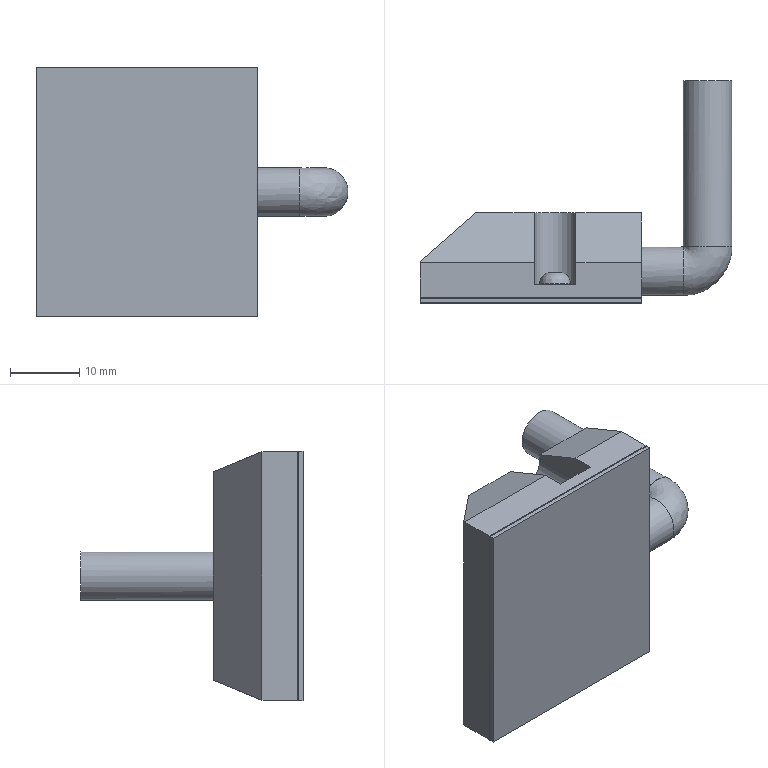Part | NX | 1 solid | 45 faces | box 45.035 x 32.1 x 36 mm | volume 14146 mm3 | plane 35 | cylinder 7 | spline 3 | commonest cylinder face diameters 4.5 x2 6 x2 7 x2 7.2 x1
STEP:
#1=CARTESIAN_POINT('',(-52.2,40.,-18.));
#2=VERTEX_POINT('',#1);
#3=CARTESIAN_POINT('',(-52.2,40.,18.));
#4=VERTEX_POINT('',#3);
#5=CARTESIAN_POINT('',(-52.2,40.,18.));
#6=DIRECTION('',(0.,0.,-1.));
#7=VECTOR('',#6,1000.);
#8=LINE('',#5,#7);
#9=EDGE_CURVE('',#2,#4,#8,.F.);
#10=ORIENTED_EDGE('',*,*,#9,.T.);
#11=CARTESIAN_POINT('',(-84.2,40.,18.));
#12=VERTEX_POINT('',#11);
#13=CARTESIAN_POINT('',(-52.2,40.,18.));
#14=DIRECTION('',(1.,0.,0.));
#15=VECTOR('',#14,1000.);
#16=LINE('',#13,#15);
#17=EDGE_CURVE('',#4,#12,#16,.F.);
#18=ORIENTED_EDGE('',*,*,#17,.T.);
#19=CARTESIAN_POINT('',(-84.2,40.,-18.));
#20=VERTEX_POINT('',#19);
#21=CARTESIAN_POINT('',(-84.2,40.,18.));
#22=DIRECTION('',(0.,0.,-1.));
#23=VECTOR('',#22,1000.);
#24=LINE('',#21,#23);
#25=EDGE_CURVE('',#12,#20,#24,.T.);
#26=ORIENTED_EDGE('',*,*,#25,.T.);
#27=CARTESIAN_POINT('',(-52.2,40.,-18.));
#28=DIRECTION('',(1.,0.,0.));
#29=VECTOR('',#28,1000.);
#30=LINE('',#27,#29);
#31=EDGE_CURVE('',#20,#2,#30,.T.);
#32=ORIENTED_EDGE('',*,*,#31,.T.);
#33=EDGE_LOOP('',(#10,#18,#26,#32));
#34=FACE_BOUND('',#33,.T.);
#35=CARTESIAN_POINT('',(-52.2,40.,18.));
#36=DIRECTION('',(0.,-1.,0.));
#37=DIRECTION('',(0.,0.,-1.));
#38=AXIS2_PLACEMENT_3D('',#35,#36,#37);
#39=PLANE('',#38);
#40=ADVANCED_FACE('',(#34),#39,.T.);
#41=CARTESIAN_POINT('',(-52.2,40.7,18.));
#42=VERTEX_POINT('',#41);
#43=CARTESIAN_POINT('',(-52.2,40.7,18.));
#44=DIRECTION('',(0.,1.,0.));
#45=VECTOR('',#44,1000.);
#46=LINE('',#43,#45);
#47=EDGE_CURVE('',#4,#42,#46,.T.);
#48=ORIENTED_EDGE('',*,*,#47,.T.);
#49=CARTESIAN_POINT('',(-84.2,40.7,18.));
#50=VERTEX_POINT('',#49);
#51=CARTESIAN_POINT('',(-52.2,40.7,18.));
#52=DIRECTION('',(1.,0.,0.));
#53=VECTOR('',#52,1000.);
#54=LINE('',#51,#53);
#55=EDGE_CURVE('',#42,#50,#54,.F.);
#56=ORIENTED_EDGE('',*,*,#55,.T.);
#57=CARTESIAN_POINT('',(-84.2,40.7,18.));
#58=DIRECTION('',(0.,1.,0.));
#59=VECTOR('',#58,1000.);
#60=LINE('',#57,#59);
#61=EDGE_CURVE('',#50,#12,#60,.F.);
#62=ORIENTED_EDGE('',*,*,#61,.T.);
#63=ORIENTED_EDGE('',*,*,#17,.F.);
#64=EDGE_LOOP('',(#48,#56,#62,#63));
#65=FACE_BOUND('',#64,.T.);
#66=CARTESIAN_POINT('',(-52.2,40.7,18.));
#67=DIRECTION('',(0.,0.,1.));
#68=DIRECTION('',(1.,0.,0.));
#69=AXIS2_PLACEMENT_3D('',#66,#67,#68);
#70=PLANE('',#69);
#71=ADVANCED_FACE('',(#65),#70,.T.);
#72=ORIENTED_EDGE('',*,*,#47,.F.);
#73=ORIENTED_EDGE('',*,*,#9,.F.);
#74=CARTESIAN_POINT('',(-52.2,40.7,-18.));
#75=VERTEX_POINT('',#74);
#76=CARTESIAN_POINT('',(-52.2,40.,-18.));
#77=DIRECTION('',(0.,1.,0.));
#78=VECTOR('',#77,1000.);
#79=LINE('',#76,#78);
#80=EDGE_CURVE('',#75,#2,#79,.F.);
#81=ORIENTED_EDGE('',*,*,#80,.F.);
#82=CARTESIAN_POINT('',(-52.2,40.7,0.));
#83=DIRECTION('',(0.,0.,1.));
#84=VECTOR('',#83,1000.);
#85=LINE('',#82,#84);
#86=EDGE_CURVE('',#42,#75,#85,.F.);
#87=ORIENTED_EDGE('',*,*,#86,.F.);
#88=EDGE_LOOP('',(#72,#73,#81,#87));
#89=FACE_BOUND('',#88,.T.);
#90=CARTESIAN_POINT('',(-52.2,40.,0.));
#91=DIRECTION('',(-1.,0.,0.));
#92=DIRECTION('',(0.,0.,1.));
#93=AXIS2_PLACEMENT_3D('',#90,#91,#92);
#94=PLANE('',#93);
#95=ADVANCED_FACE('',(#89),#94,.F.);
#96=ORIENTED_EDGE('',*,*,#80,.T.);
#97=ORIENTED_EDGE('',*,*,#31,.F.);
#98=CARTESIAN_POINT('',(-84.2,40.7,-18.));
#99=VERTEX_POINT('',#98);
#100=CARTESIAN_POINT('',(-84.2,40.,-18.));
#101=DIRECTION('',(0.,1.,0.));
#102=VECTOR('',#101,1000.);
#103=LINE('',#100,#102);
#104=EDGE_CURVE('',#20,#99,#103,.T.);
#105=ORIENTED_EDGE('',*,*,#104,.T.);
#106=CARTESIAN_POINT('',(-52.2,40.7,-18.));
#107=DIRECTION('',(-1.,0.,0.));
#108=VECTOR('',#107,1000.);
#109=LINE('',#106,#108);
#110=EDGE_CURVE('',#99,#75,#109,.F.);
#111=ORIENTED_EDGE('',*,*,#110,.T.);
#112=EDGE_LOOP('',(#96,#97,#105,#111));
#113=FACE_BOUND('',#112,.T.);
#114=CARTESIAN_POINT('',(-52.2,40.,-18.));
#115=DIRECTION('',(0.,0.,-1.));
#116=DIRECTION('',(-1.,0.,0.));
#117=AXIS2_PLACEMENT_3D('',#114,#115,#116);
#118=PLANE('',#117);
#119=ADVANCED_FACE('',(#113),#118,.T.);
#120=ORIENTED_EDGE('',*,*,#25,.F.);
#121=ORIENTED_EDGE('',*,*,#61,.F.);
#122=CARTESIAN_POINT('',(-84.2,40.7,0.));
#123=DIRECTION('',(0.,0.,1.));
#124=VECTOR('',#123,1000.);
#125=LINE('',#122,#124);
#126=EDGE_CURVE('',#50,#99,#125,.F.);
#127=ORIENTED_EDGE('',*,*,#126,.T.);
#128=ORIENTED_EDGE('',*,*,#104,.F.);
#129=EDGE_LOOP('',(#120,#121,#127,#128));
#130=FACE_BOUND('',#129,.T.);
#131=CARTESIAN_POINT('',(-84.2,40.,0.));
#132=DIRECTION('',(-1.,0.,0.));
#133=DIRECTION('',(0.,0.,1.));
#134=AXIS2_PLACEMENT_3D('',#131,#132,#133);
#135=PLANE('',#134);
#136=ADVANCED_FACE('',(#130),#135,.T.);
#137=ORIENTED_EDGE('',*,*,#86,.T.);
#138=ORIENTED_EDGE('',*,*,#110,.F.);
#139=ORIENTED_EDGE('',*,*,#126,.F.);
#140=ORIENTED_EDGE('',*,*,#55,.F.);
#141=EDGE_LOOP('',(#137,#138,#139,#140));
#142=FACE_BOUND('',#141,.T.);
#143=CARTESIAN_POINT('',(-52.3,40.7,17.9));
#144=VERTEX_POINT('',#143);
#145=CARTESIAN_POINT('',(-84.1,40.7,17.9));
#146=VERTEX_POINT('',#145);
#147=CARTESIAN_POINT('',(-52.2,40.7,17.9));
#148=DIRECTION('',(1.,0.,0.));
#149=VECTOR('',#148,1000.);
#150=LINE('',#147,#149);
#151=EDGE_CURVE('',#144,#146,#150,.F.);
#152=ORIENTED_EDGE('',*,*,#151,.T.);
#153=CARTESIAN_POINT('',(-84.1,40.7,-17.9));
#154=VERTEX_POINT('',#153);
#155=CARTESIAN_POINT('',(-84.1,40.7,-18.));
#156=DIRECTION('',(0.,0.,1.));
#157=VECTOR('',#156,1000.);
#158=LINE('',#155,#157);
#159=EDGE_CURVE('',#146,#154,#158,.F.);
#160=ORIENTED_EDGE('',*,*,#159,.T.);
#161=CARTESIAN_POINT('',(-52.3,40.7,-17.9));
#162=VERTEX_POINT('',#161);
#163=CARTESIAN_POINT('',(-52.2,40.7,-17.9));
#164=DIRECTION('',(1.,0.,0.));
#165=VECTOR('',#164,1000.);
#166=LINE('',#163,#165);
#167=EDGE_CURVE('',#154,#162,#166,.T.);
#168=ORIENTED_EDGE('',*,*,#167,.T.);
#169=CARTESIAN_POINT('',(-52.3,40.7,-18.));
#170=DIRECTION('',(0.,0.,1.));
#171=VECTOR('',#170,1000.);
#172=LINE('',#169,#171);
#173=EDGE_CURVE('',#162,#144,#172,.T.);
#174=ORIENTED_EDGE('',*,*,#173,.T.);
#175=EDGE_LOOP('',(#152,#160,#168,#174));
#176=FACE_BOUND('',#175,.T.);
#177=CARTESIAN_POINT('',(-52.2,40.7,-18.));
#178=DIRECTION('',(0.,1.,0.));
#179=DIRECTION('',(0.,0.,1.));
#180=AXIS2_PLACEMENT_3D('',#177,#178,#179);
#181=PLANE('',#180);
#182=ADVANCED_FACE('',(#142,#176),#181,.T.);
#183=CARTESIAN_POINT('',(-84.1,40.8,17.9));
#184=VERTEX_POINT('',#183);
#185=CARTESIAN_POINT('',(-84.1,40.,17.9));
#186=DIRECTION('',(0.,1.,0.));
#187=VECTOR('',#186,1000.);
#188=LINE('',#185,#187);
#189=EDGE_CURVE('',#146,#184,#188,.T.);
#190=ORIENTED_EDGE('',*,*,#189,.T.);
#191=CARTESIAN_POINT('',(-84.1,40.8,-17.9));
#192=VERTEX_POINT('',#191);
#193=CARTESIAN_POINT('',(-84.1,40.8,0.));
#194=DIRECTION('',(0.,0.,1.));
#195=VECTOR('',#194,1000.);
#196=LINE('',#193,#195);
#197=EDGE_CURVE('',#184,#192,#196,.F.);
#198=ORIENTED_EDGE('',*,*,#197,.T.);
#199=CARTESIAN_POINT('',(-84.1,40.,-17.9));
#200=DIRECTION('',(0.,1.,0.));
#201=VECTOR('',#200,1000.);
#202=LINE('',#199,#201);
#203=EDGE_CURVE('',#192,#154,#202,.F.);
#204=ORIENTED_EDGE('',*,*,#203,.T.);
#205=ORIENTED_EDGE('',*,*,#159,.F.);
#206=EDGE_LOOP('',(#190,#198,#204,#205));
#207=FACE_BOUND('',#206,.T.);
#208=CARTESIAN_POINT('',(-84.1,40.,0.));
#209=DIRECTION('',(-1.,0.,0.));
#210=DIRECTION('',(0.,0.,1.));
#211=AXIS2_PLACEMENT_3D('',#208,#209,#210);
#212=PLANE('',#211);
#213=ADVANCED_FACE('',(#207),#212,.T.);
#214=CARTESIAN_POINT('',(-52.3,40.8,17.9));
#215=VERTEX_POINT('',#214);
#216=CARTESIAN_POINT('',(-52.3,40.8,17.9));
#217=DIRECTION('',(0.,1.,0.));
#218=VECTOR('',#217,1000.);
#219=LINE('',#216,#218);
#220=EDGE_CURVE('',#144,#215,#219,.T.);
#221=ORIENTED_EDGE('',*,*,#220,.T.);
#222=CARTESIAN_POINT('',(-52.2,40.8,17.9));
#223=DIRECTION('',(1.,0.,0.));
#224=VECTOR('',#223,1000.);
#225=LINE('',#222,#224);
#226=EDGE_CURVE('',#215,#184,#225,.F.);
#227=ORIENTED_EDGE('',*,*,#226,.T.);
#228=ORIENTED_EDGE('',*,*,#189,.F.);
#229=ORIENTED_EDGE('',*,*,#151,.F.);
#230=EDGE_LOOP('',(#221,#227,#228,#229));
#231=FACE_BOUND('',#230,.T.);
#232=CARTESIAN_POINT('',(-52.2,40.8,17.9));
#233=DIRECTION('',(0.,0.,1.));
#234=DIRECTION('',(1.,0.,0.));
#235=AXIS2_PLACEMENT_3D('',#232,#233,#234);
#236=PLANE('',#235);
#237=ADVANCED_FACE('',(#231),#236,.T.);
#238=CARTESIAN_POINT('',(-52.3,40.8,-3.6));
#239=VERTEX_POINT('',#238);
#240=CARTESIAN_POINT('',(-52.3,40.8,-17.9));
#241=VERTEX_POINT('',#240);
#242=CARTESIAN_POINT('',(-52.3,40.8,0.));
#243=DIRECTION('',(0.,0.,1.));
#244=VECTOR('',#243,1000.);
#245=LINE('',#242,#244);
#246=EDGE_CURVE('',#239,#241,#245,.F.);
#247=ORIENTED_EDGE('',*,*,#246,.F.);
#248=CARTESIAN_POINT('',(-52.3,44.6,-3.6));
#249=VERTEX_POINT('',#248);
#250=CARTESIAN_POINT('',(-52.3,40.,-3.6));
#251=DIRECTION('',(0.,1.,0.));
#252=VECTOR('',#251,1000.);
#253=LINE('',#250,#252);
#254=EDGE_CURVE('',#249,#239,#253,.F.);
#255=ORIENTED_EDGE('',*,*,#254,.F.);
#256=CARTESIAN_POINT('',(-52.3,44.6,3.6));
#257=VERTEX_POINT('',#256);
#258=CARTESIAN_POINT('',(-52.3,44.6,0.));
#259=DIRECTION('',(1.,0.,0.));
#260=DIRECTION('',(0.,0.,-1.));
#261=AXIS2_PLACEMENT_3D('',#258,#259,#260);
#262=CIRCLE('',#261,3.6);
#263=EDGE_CURVE('',#257,#249,#262,.F.);
#264=ORIENTED_EDGE('',*,*,#263,.F.);
#265=CARTESIAN_POINT('',(-52.3,40.8,3.6));
#266=VERTEX_POINT('',#265);
#267=CARTESIAN_POINT('',(-52.3,40.,3.6));
#268=DIRECTION('',(0.,1.,0.));
#269=VECTOR('',#268,1000.);
#270=LINE('',#267,#269);
#271=EDGE_CURVE('',#266,#257,#270,.T.);
#272=ORIENTED_EDGE('',*,*,#271,.F.);
#273=CARTESIAN_POINT('',(-52.3,40.8,0.));
#274=DIRECTION('',(0.,0.,1.));
#275=VECTOR('',#274,1000.);
#276=LINE('',#273,#275);
#277=EDGE_CURVE('',#215,#266,#276,.F.);
#278=ORIENTED_EDGE('',*,*,#277,.F.);
#279=ORIENTED_EDGE('',*,*,#220,.F.);
#280=ORIENTED_EDGE('',*,*,#173,.F.);
#281=CARTESIAN_POINT('',(-52.3,40.,-17.9));
#282=DIRECTION('',(0.,1.,0.));
#283=VECTOR('',#282,1000.);
#284=LINE('',#281,#283);
#285=EDGE_CURVE('',#241,#162,#284,.F.);
#286=ORIENTED_EDGE('',*,*,#285,.F.);
#287=EDGE_LOOP('',(#247,#255,#264,#272,#278,#279,#280,#286));
#288=FACE_BOUND('',#287,.T.);
#289=CARTESIAN_POINT('',(-52.3,44.6,-3.5));
#290=VERTEX_POINT('',#289);
#291=CARTESIAN_POINT('',(-52.3,44.6,0.));
#292=DIRECTION('',(1.,0.,0.));
#293=DIRECTION('',(0.,0.,-1.));
#294=AXIS2_PLACEMENT_3D('',#291,#292,#293);
#295=CIRCLE('',#294,3.5);
#296=EDGE_CURVE('',#290,#290,#295,.T.);
#297=ORIENTED_EDGE('',*,*,#296,.F.);
#298=EDGE_LOOP('',(#297));
#299=FACE_BOUND('',#298,.T.);
#300=CARTESIAN_POINT('',(-52.3,40.,0.));
#301=DIRECTION('',(-1.,0.,0.));
#302=DIRECTION('',(0.,0.,1.));
#303=AXIS2_PLACEMENT_3D('',#300,#301,#302);
#304=PLANE('',#303);
#305=ADVANCED_FACE('',(#288,#299),#304,.F.);
#306=ORIENTED_EDGE('',*,*,#285,.T.);
#307=ORIENTED_EDGE('',*,*,#167,.F.);
#308=ORIENTED_EDGE('',*,*,#203,.F.);
#309=CARTESIAN_POINT('',(-52.2,40.8,-17.9));
#310=DIRECTION('',(1.,0.,0.));
#311=VECTOR('',#310,1000.);
#312=LINE('',#309,#311);
#313=EDGE_CURVE('',#192,#241,#312,.T.);
#314=ORIENTED_EDGE('',*,*,#313,.T.);
#315=EDGE_LOOP('',(#306,#307,#308,#314));
#316=FACE_BOUND('',#315,.T.);
#317=CARTESIAN_POINT('',(-52.2,40.7,-17.9));
#318=DIRECTION('',(0.,0.,-1.));
#319=DIRECTION('',(0.,1.,0.));
#320=AXIS2_PLACEMENT_3D('',#317,#318,#319);
#321=PLANE('',#320);
#322=ADVANCED_FACE('',(#316),#321,.T.);
#323=CARTESIAN_POINT('',(-84.2,40.8,-18.));
#324=VERTEX_POINT('',#323);
#325=CARTESIAN_POINT('',(-52.2,40.8,-18.));
#326=VERTEX_POINT('',#325);
#327=CARTESIAN_POINT('',(-52.2,40.8,-18.));
#328=DIRECTION('',(1.,0.,0.));
#329=VECTOR('',#328,1000.);
#330=LINE('',#327,#329);
#331=EDGE_CURVE('',#324,#326,#330,.T.);
#332=ORIENTED_EDGE('',*,*,#331,.T.);
#333=CARTESIAN_POINT('',(-52.2,40.8,-3.6));
#334=VERTEX_POINT('',#333);
#335=CARTESIAN_POINT('',(-52.2,40.8,-17.9));
#336=DIRECTION('',(0.,0.,-1.));
#337=VECTOR('',#336,1000.);
#338=LINE('',#335,#337);
#339=EDGE_CURVE('',#326,#334,#338,.F.);
#340=ORIENTED_EDGE('',*,*,#339,.T.);
#341=CARTESIAN_POINT('',(-52.2,40.8,-3.6));
#342=DIRECTION('',(1.,0.,0.));
#343=VECTOR('',#342,1000.);
#344=LINE('',#341,#343);
#345=EDGE_CURVE('',#334,#239,#344,.F.);
#346=ORIENTED_EDGE('',*,*,#345,.T.);
#347=ORIENTED_EDGE('',*,*,#246,.T.);
#348=ORIENTED_EDGE('',*,*,#313,.F.);
#349=ORIENTED_EDGE('',*,*,#197,.F.);
#350=ORIENTED_EDGE('',*,*,#226,.F.);
#351=ORIENTED_EDGE('',*,*,#277,.T.);
#352=CARTESIAN_POINT('',(-52.2,40.8,3.6));
#353=VERTEX_POINT('',#352);
#354=CARTESIAN_POINT('',(-52.2,40.8,3.6));
#355=DIRECTION('',(1.,0.,0.));
#356=VECTOR('',#355,1000.);
#357=LINE('',#354,#356);
#358=EDGE_CURVE('',#266,#353,#357,.T.);
#359=ORIENTED_EDGE('',*,*,#358,.T.);
#360=CARTESIAN_POINT('',(-52.2,40.8,18.));
#361=VERTEX_POINT('',#360);
#362=CARTESIAN_POINT('',(-52.2,40.8,-17.9));
#363=DIRECTION('',(0.,0.,-1.));
#364=VECTOR('',#363,1000.);
#365=LINE('',#362,#364);
#366=EDGE_CURVE('',#353,#361,#365,.F.);
#367=ORIENTED_EDGE('',*,*,#366,.T.);
#368=CARTESIAN_POINT('',(-84.2,40.8,18.));
#369=VERTEX_POINT('',#368);
#370=CARTESIAN_POINT('',(-52.2,40.8,18.));
#371=DIRECTION('',(1.,0.,0.));
#372=VECTOR('',#371,1000.);
#373=LINE('',#370,#372);
#374=EDGE_CURVE('',#361,#369,#373,.F.);
#375=ORIENTED_EDGE('',*,*,#374,.T.);
#376=CARTESIAN_POINT('',(-84.2,40.8,-17.9));
#377=DIRECTION('',(0.,0.,-1.));
#378=VECTOR('',#377,1000.);
#379=LINE('',#376,#378);
#380=EDGE_CURVE('',#369,#324,#379,.T.);
#381=ORIENTED_EDGE('',*,*,#380,.T.);
#382=EDGE_LOOP('',(#332,#340,#346,#347,#348,#349,#350,#351,#359,#367,#375,#381));
#383=FACE_BOUND('',#382,.T.);
#384=CARTESIAN_POINT('',(-52.2,40.8,-17.9));
#385=DIRECTION('',(0.,-1.,0.));
#386=DIRECTION('',(0.,0.,-1.));
#387=AXIS2_PLACEMENT_3D('',#384,#385,#386);
#388=PLANE('',#387);
#389=ADVANCED_FACE('',(#383),#388,.T.);
#390=ORIENTED_EDGE('',*,*,#345,.F.);
#391=CARTESIAN_POINT('',(-52.2,44.6,-3.6));
#392=VERTEX_POINT('',#391);
#393=CARTESIAN_POINT('',(-52.2,40.8,-3.6));
#394=DIRECTION('',(0.,1.,0.));
#395=VECTOR('',#394,1000.);
#396=LINE('',#393,#395);
#397=EDGE_CURVE('',#392,#334,#396,.F.);
#398=ORIENTED_EDGE('',*,*,#397,.F.);
#399=CARTESIAN_POINT('',(-52.2,44.6,-3.6));
#400=DIRECTION('',(-1.,0.,0.));
#401=VECTOR('',#400,1000.);
#402=LINE('',#399,#401);
#403=EDGE_CURVE('',#249,#392,#402,.F.);
#404=ORIENTED_EDGE('',*,*,#403,.F.);
#405=ORIENTED_EDGE('',*,*,#254,.T.);
#406=EDGE_LOOP('',(#390,#398,#404,#405));
#407=FACE_BOUND('',#406,.T.);
#408=CARTESIAN_POINT('',(-52.2,40.8,-3.6));
#409=DIRECTION('',(0.,0.,-1.));
#410=DIRECTION('',(-1.,0.,0.));
#411=AXIS2_PLACEMENT_3D('',#408,#409,#410);
#412=PLANE('',#411);
#413=ADVANCED_FACE('',(#407),#412,.F.);
#414=ORIENTED_EDGE('',*,*,#403,.T.);
#415=CARTESIAN_POINT('',(-52.2,44.6,3.6));
#416=VERTEX_POINT('',#415);
#417=CARTESIAN_POINT('',(-52.2,44.6,0.));
#418=DIRECTION('',(1.,0.,0.));
#419=DIRECTION('',(0.,0.,-1.));
#420=AXIS2_PLACEMENT_3D('',#417,#418,#419);
#421=CIRCLE('',#420,3.6);
#422=EDGE_CURVE('',#416,#392,#421,.F.);
#423=ORIENTED_EDGE('',*,*,#422,.F.);
#424=CARTESIAN_POINT('',(-52.2,44.6,3.6));
#425=DIRECTION('',(1.,0.,0.));
#426=VECTOR('',#425,1000.);
#427=LINE('',#424,#426);
#428=EDGE_CURVE('',#257,#416,#427,.T.);
#429=ORIENTED_EDGE('',*,*,#428,.F.);
#430=ORIENTED_EDGE('',*,*,#263,.T.);
#431=EDGE_LOOP('',(#414,#423,#429,#430));
#432=FACE_BOUND('',#431,.T.);
#433=CARTESIAN_POINT('',(-52.2,44.6,0.));
#434=DIRECTION('',(1.,0.,0.));
#435=DIRECTION('',(0.,0.,-1.));
#436=AXIS2_PLACEMENT_3D('',#433,#434,#435);
#437=CYLINDRICAL_SURFACE('',#436,3.6);
#438=ADVANCED_FACE('',(#432),#437,.F.);
#439=ORIENTED_EDGE('',*,*,#428,.T.);
#440=CARTESIAN_POINT('',(-52.2,44.6,3.6));
#441=DIRECTION('',(0.,1.,0.));
#442=VECTOR('',#441,1000.);
#443=LINE('',#440,#442);
#444=EDGE_CURVE('',#353,#416,#443,.T.);
#445=ORIENTED_EDGE('',*,*,#444,.F.);
#446=ORIENTED_EDGE('',*,*,#358,.F.);
#447=ORIENTED_EDGE('',*,*,#271,.T.);
#448=EDGE_LOOP('',(#439,#445,#446,#447));
#449=FACE_BOUND('',#448,.T.);
#450=CARTESIAN_POINT('',(-52.2,44.6,3.6));
#451=DIRECTION('',(0.,0.,1.));
#452=DIRECTION('',(1.,0.,0.));
#453=AXIS2_PLACEMENT_3D('',#450,#451,#452);
#454=PLANE('',#453);
#455=ADVANCED_FACE('',(#449),#454,.F.);
#456=CARTESIAN_POINT('',(-46.2,48.1,0.));
#457=VERTEX_POINT('',#456);
#458=CARTESIAN_POINT('',(-46.2,44.6,0.));
#459=DIRECTION('',(1.,0.,0.));
#460=DIRECTION('',(0.,0.,-1.));
#461=AXIS2_PLACEMENT_3D('',#458,#459,#460);
#462=CIRCLE('',#461,3.5);
#463=EDGE_CURVE('',#457,#457,#462,.F.);
#464=ORIENTED_EDGE('',*,*,#463,.T.);
#465=EDGE_LOOP('',(#464));
#466=FACE_BOUND('',#465,.T.);
#467=ORIENTED_EDGE('',*,*,#296,.T.);
#468=EDGE_LOOP('',(#467));
#469=FACE_BOUND('',#468,.T.);
#470=CARTESIAN_POINT('',(-46.2,44.6,0.));
#471=DIRECTION('',(1.,0.,0.));
#472=DIRECTION('',(0.,0.,-1.));
#473=AXIS2_PLACEMENT_3D('',#470,#471,#472);
#474=CYLINDRICAL_SURFACE('',#473,3.5);
#475=ADVANCED_FACE('',(#466,#469),#474,.T.);
#476=ORIENTED_EDGE('',*,*,#339,.F.);
#477=CARTESIAN_POINT('',(-52.2,45.8,-18.));
#478=VERTEX_POINT('',#477);
#479=CARTESIAN_POINT('',(-52.2,40.,-18.));
#480=DIRECTION('',(0.,1.,0.));
#481=VECTOR('',#480,1000.);
#482=LINE('',#479,#481);
#483=EDGE_CURVE('',#478,#326,#482,.F.);
#484=ORIENTED_EDGE('',*,*,#483,.F.);
#485=CARTESIAN_POINT('',(-52.2,53.,-15.041));
#486=VERTEX_POINT('',#485);
#487=CARTESIAN_POINT('',(-52.2,53.,-15.041));
#488=DIRECTION('',(0.,-0.9249,-0.3801));
#489=VECTOR('',#488,1000.);
#490=LINE('',#487,#489);
#491=EDGE_CURVE('',#486,#478,#490,.T.);
#492=ORIENTED_EDGE('',*,*,#491,.F.);
#493=CARTESIAN_POINT('',(-52.2,53.,15.041));
#494=VERTEX_POINT('',#493);
#495=CARTESIAN_POINT('',(-52.2,53.,0.));
#496=DIRECTION('',(0.,0.,1.));
#497=VECTOR('',#496,1000.);
#498=LINE('',#495,#497);
#499=EDGE_CURVE('',#494,#486,#498,.F.);
#500=ORIENTED_EDGE('',*,*,#499,.F.);
#501=CARTESIAN_POINT('',(-52.2,45.8,18.));
#502=VERTEX_POINT('',#501);
#503=CARTESIAN_POINT('',(-52.2,45.8,18.));
#504=DIRECTION('',(0.,0.9249,-0.3801));
#505=VECTOR('',#504,1000.);
#506=LINE('',#503,#505);
#507=EDGE_CURVE('',#502,#494,#506,.T.);
#508=ORIENTED_EDGE('',*,*,#507,.F.);
#509=CARTESIAN_POINT('',(-52.2,40.,18.));
#510=DIRECTION('',(0.,1.,0.));
#511=VECTOR('',#510,1000.);
#512=LINE('',#509,#511);
#513=EDGE_CURVE('',#361,#502,#512,.T.);
#514=ORIENTED_EDGE('',*,*,#513,.F.);
#515=ORIENTED_EDGE('',*,*,#366,.F.);
#516=ORIENTED_EDGE('',*,*,#444,.T.);
#517=ORIENTED_EDGE('',*,*,#422,.T.);
#518=ORIENTED_EDGE('',*,*,#397,.T.);
#519=EDGE_LOOP('',(#476,#484,#492,#500,#508,#514,#515,#516,#517,#518));
#520=FACE_BOUND('',#519,.T.);
#521=CARTESIAN_POINT('',(-52.2,40.,0.));
#522=DIRECTION('',(-1.,0.,0.));
#523=DIRECTION('',(0.,0.,1.));
#524=AXIS2_PLACEMENT_3D('',#521,#522,#523);
#525=PLANE('',#524);
#526=ADVANCED_FACE('',(#520),#525,.F.);
#527=CARTESIAN_POINT('',(-67.7,45.8,-18.));
#528=VERTEX_POINT('',#527);
#529=CARTESIAN_POINT('',(-67.7,42.7,-18.));
#530=VERTEX_POINT('',#529);
#531=CARTESIAN_POINT('',(-67.7,40.8,-18.));
#532=DIRECTION('',(0.,1.,0.));
#533=VECTOR('',#532,1000.);
#534=LINE('',#531,#533);
#535=EDGE_CURVE('',#528,#530,#534,.F.);
#536=ORIENTED_EDGE('',*,*,#535,.T.);
#537=CARTESIAN_POINT('',(-61.7,42.7,-18.));
#538=VERTEX_POINT('',#537);
#539=CARTESIAN_POINT('',(-52.2,42.7,-18.));
#540=DIRECTION('',(-1.,0.,0.));
#541=VECTOR('',#540,1000.);
#542=LINE('',#539,#541);
#543=EDGE_CURVE('',#530,#538,#542,.F.);
#544=ORIENTED_EDGE('',*,*,#543,.T.);
#545=CARTESIAN_POINT('',(-61.7,45.8,-18.));
#546=VERTEX_POINT('',#545);
#547=CARTESIAN_POINT('',(-61.7,40.8,-18.));
#548=DIRECTION('',(0.,1.,0.));
#549=VECTOR('',#548,1000.);
#550=LINE('',#547,#549);
#551=EDGE_CURVE('',#538,#546,#550,.T.);
#552=ORIENTED_EDGE('',*,*,#551,.T.);
#553=CARTESIAN_POINT('',(-52.2,45.8,-18.));
#554=DIRECTION('',(-1.,0.,0.));
#555=VECTOR('',#554,1000.);
#556=LINE('',#553,#555);
#557=EDGE_CURVE('',#546,#478,#556,.F.);
#558=ORIENTED_EDGE('',*,*,#557,.T.);
#559=ORIENTED_EDGE('',*,*,#483,.T.);
#560=ORIENTED_EDGE('',*,*,#331,.F.);
#561=CARTESIAN_POINT('',(-84.2,45.8,-18.));
#562=VERTEX_POINT('',#561);
#563=CARTESIAN_POINT('',(-84.2,40.8,-18.));
#564=DIRECTION('',(0.,1.,0.));
#565=VECTOR('',#564,1000.);
#566=LINE('',#563,#565);
#567=EDGE_CURVE('',#324,#562,#566,.T.);
#568=ORIENTED_EDGE('',*,*,#567,.T.);
#569=CARTESIAN_POINT('',(-52.2,45.8,-18.));
#570=DIRECTION('',(-1.,0.,0.));
#571=VECTOR('',#570,1000.);
#572=LINE('',#569,#571);
#573=EDGE_CURVE('',#562,#528,#572,.F.);
#574=ORIENTED_EDGE('',*,*,#573,.T.);
#575=EDGE_LOOP('',(#536,#544,#552,#558,#559,#560,#568,#574));
#576=FACE_BOUND('',#575,.T.);
#577=CARTESIAN_POINT('',(-52.2,40.8,-18.));
#578=DIRECTION('',(0.,0.,-1.));
#579=DIRECTION('',(-1.,0.,0.));
#580=AXIS2_PLACEMENT_3D('',#577,#578,#579);
#581=PLANE('',#580);
#582=ADVANCED_FACE('',(#576),#581,.T.);
#583=CARTESIAN_POINT('',(-84.2,45.8,18.));
#584=VERTEX_POINT('',#583);
#585=CARTESIAN_POINT('',(-84.2,40.,18.));
#586=DIRECTION('',(0.,1.,0.));
#587=VECTOR('',#586,1000.);
#588=LINE('',#585,#587);
#589=EDGE_CURVE('',#369,#584,#588,.T.);
#590=ORIENTED_EDGE('',*,*,#589,.T.);
#591=CARTESIAN_POINT('',(-84.2,46.,17.918));
#592=VERTEX_POINT('',#591);
#593=CARTESIAN_POINT('',(-84.2,53.,15.041));
#594=DIRECTION('',(0.,-0.9249,0.3801));
#595=VECTOR('',#594,1000.);
#596=LINE('',#593,#595);
#597=EDGE_CURVE('',#592,#584,#596,.T.);
#598=ORIENTED_EDGE('',*,*,#597,.F.);
#599=CARTESIAN_POINT('',(-84.2,46.,-17.918));
#600=VERTEX_POINT('',#599);
#601=CARTESIAN_POINT('',(-84.2,46.,0.));
#602=DIRECTION('',(0.,0.,1.));
#603=VECTOR('',#602,1000.);
#604=LINE('',#601,#603);
#605=EDGE_CURVE('',#592,#600,#604,.F.);
#606=ORIENTED_EDGE('',*,*,#605,.T.);
#607=CARTESIAN_POINT('',(-84.2,46.,-17.918));
#608=DIRECTION('',(0.,-0.9249,-0.3801));
#609=VECTOR('',#608,1000.);
#610=LINE('',#607,#609);
#611=EDGE_CURVE('',#600,#562,#610,.T.);
#612=ORIENTED_EDGE('',*,*,#611,.T.);
#613=ORIENTED_EDGE('',*,*,#567,.F.);
#614=ORIENTED_EDGE('',*,*,#380,.F.);
#615=EDGE_LOOP('',(#590,#598,#606,#612,#613,#614));
#616=FACE_BOUND('',#615,.T.);
#617=CARTESIAN_POINT('',(-84.2,40.,0.));
#618=DIRECTION('',(-1.,0.,0.));
#619=DIRECTION('',(0.,0.,1.));
#620=AXIS2_PLACEMENT_3D('',#617,#618,#619);
#621=PLANE('',#620);
#622=ADVANCED_FACE('',(#616),#621,.T.);
#623=CARTESIAN_POINT('',(-61.7,45.8,18.));
#624=VERTEX_POINT('',#623);
#625=CARTESIAN_POINT('',(-61.7,42.7,18.));
#626=VERTEX_POINT('',#625);
#627=CARTESIAN_POINT('',(-61.7,45.8,18.));
#628=DIRECTION('',(0.,1.,0.));
#629=VECTOR('',#628,1000.);
#630=LINE('',#627,#629);
#631=EDGE_CURVE('',#624,#626,#630,.F.);
#632=ORIENTED_EDGE('',*,*,#631,.T.);
#633=CARTESIAN_POINT('',(-67.7,42.7,18.));
#634=VERTEX_POINT('',#633);
#635=CARTESIAN_POINT('',(-52.2,42.7,18.));
#636=DIRECTION('',(1.,0.,0.));
#637=VECTOR('',#636,1000.);
#638=LINE('',#635,#637);
#639=EDGE_CURVE('',#626,#634,#638,.F.);
#640=ORIENTED_EDGE('',*,*,#639,.T.);
#641=CARTESIAN_POINT('',(-67.7,45.8,18.));
#642=VERTEX_POINT('',#641);
#643=CARTESIAN_POINT('',(-67.7,45.8,18.));
#644=DIRECTION('',(0.,1.,0.));
#645=VECTOR('',#644,1000.);
#646=LINE('',#643,#645);
#647=EDGE_CURVE('',#634,#642,#646,.T.);
#648=ORIENTED_EDGE('',*,*,#647,.T.);
#649=CARTESIAN_POINT('',(-52.2,45.8,18.));
#650=DIRECTION('',(1.,0.,0.));
#651=VECTOR('',#650,1000.);
#652=LINE('',#649,#651);
#653=EDGE_CURVE('',#642,#584,#652,.F.);
#654=ORIENTED_EDGE('',*,*,#653,.T.);
#655=ORIENTED_EDGE('',*,*,#589,.F.);
#656=ORIENTED_EDGE('',*,*,#374,.F.);
#657=ORIENTED_EDGE('',*,*,#513,.T.);
#658=CARTESIAN_POINT('',(-52.2,45.8,18.));
#659=DIRECTION('',(1.,0.,0.));
#660=VECTOR('',#659,1000.);
#661=LINE('',#658,#660);
#662=EDGE_CURVE('',#502,#624,#661,.F.);
#663=ORIENTED_EDGE('',*,*,#662,.T.);
#664=EDGE_LOOP('',(#632,#640,#648,#654,#655,#656,#657,#663));
#665=FACE_BOUND('',#664,.T.);
#666=CARTESIAN_POINT('',(-52.2,45.8,18.));
#667=DIRECTION('',(0.,0.,1.));
#668=DIRECTION('',(1.,0.,0.));
#669=AXIS2_PLACEMENT_3D('',#666,#667,#668);
#670=PLANE('',#669);
#671=ADVANCED_FACE('',(#665),#670,.T.);
#672=CARTESIAN_POINT('',(-42.682,48.135,-3.5));
#673=VERTEX_POINT('',#672);
#674=CARTESIAN_POINT('',(-42.691,48.1,-3.5));
#675=VERTEX_POINT('',#674);
#676=CARTESIAN_POINT('',(-42.682,48.135,-3.5));
#677=CARTESIAN_POINT('',(-42.683,48.123,-3.5));
#678=CARTESIAN_POINT('',(-42.683,48.112,-3.5));
#679=CARTESIAN_POINT('',(-42.683,48.1,-3.5));
#680=B_SPLINE_CURVE_WITH_KNOTS('',3,(#676,#677,#678,#679),.UNSPECIFIED.,.F.,.F.,(4,4),(0.,1.),.UNSPECIFIED.);
#681=EDGE_CURVE('',#673,#675,#680,.T.);
#682=ORIENTED_EDGE('',*,*,#681,.F.);
#683=CARTESIAN_POINT('',(-42.682,48.135,3.5));
#684=VERTEX_POINT('',#683);
#685=CARTESIAN_POINT('',(-42.682,48.135,-3.5));
#686=CARTESIAN_POINT('',(-41.755,48.135,-3.505));
#687=CARTESIAN_POINT('',(-39.934,48.135,-2.753));
#688=CARTESIAN_POINT('',(-38.781,48.135,0.0008832));
#689=CARTESIAN_POINT('',(-39.931,48.135,2.749));
#690=CARTESIAN_POINT('',(-41.755,48.135,3.505));
#691=CARTESIAN_POINT('',(-42.682,48.135,3.5));
#692=B_SPLINE_CURVE_WITH_KNOTS('',3,(#685,#686,#687,#688,#689,#690,#691),.UNSPECIFIED.,.F.,.F.,(4,1,1,1,4),(0.,0.002743,0.005485,0.008228,0.01097),.UNSPECIFIED.);
#693=EDGE_CURVE('',#673,#684,#692,.T.);
#694=ORIENTED_EDGE('',*,*,#693,.T.);
#695=CARTESIAN_POINT('',(-42.691,48.1,3.5));
#696=VERTEX_POINT('',#695);
#697=CARTESIAN_POINT('',(-42.683,48.1,3.5));
#698=CARTESIAN_POINT('',(-42.683,48.112,3.5));
#699=CARTESIAN_POINT('',(-42.683,48.123,3.5));
#700=CARTESIAN_POINT('',(-42.683,48.135,3.5));
#701=B_SPLINE_CURVE_WITH_KNOTS('',3,(#697,#698,#699,#700),.UNSPECIFIED.,.F.,.F.,(4,4),(0.,1.),.UNSPECIFIED.);
#702=EDGE_CURVE('',#696,#684,#701,.T.);
#703=ORIENTED_EDGE('',*,*,#702,.F.);
#704=CARTESIAN_POINT('',(-42.691,48.1,3.5));
#705=CARTESIAN_POINT('',(-43.612,48.1,3.493));
#706=CARTESIAN_POINT('',(-44.952,48.1,2.916));
#707=CARTESIAN_POINT('',(-45.992,48.1,1.371));
#708=CARTESIAN_POINT('',(-46.155,48.1,0.4516));
#709=CARTESIAN_POINT('',(-46.2,48.1,0.));
#710=B_SPLINE_CURVE_WITH_KNOTS('',3,(#704,#705,#706,#707,#708,#709),.UNSPECIFIED.,.F.,.F.,(4,1,1,4),(0.,0.002723,0.004084,0.005446),.UNSPECIFIED.);
#711=EDGE_CURVE('',#696,#457,#710,.T.);
#712=ORIENTED_EDGE('',*,*,#711,.T.);
#713=ORIENTED_EDGE('',*,*,#463,.F.);
#714=CARTESIAN_POINT('',(-42.7,48.1,-3.5));
#715=CARTESIAN_POINT('',(-43.161,48.1,-3.495));
#716=CARTESIAN_POINT('',(-44.059,48.1,-3.306));
#717=CARTESIAN_POINT('',(-45.216,48.1,-2.529));
#718=CARTESIAN_POINT('',(-45.855,48.1,-1.557));
#719=CARTESIAN_POINT('',(-46.09,48.1,-0.8039));
#720=CARTESIAN_POINT('',(-46.169,48.1,-0.3137));
#721=CARTESIAN_POINT('',(-46.185,48.1,-0.1451));
#722=CARTESIAN_POINT('',(-46.2,48.1,0.));
#723=B_SPLINE_CURVE_WITH_KNOTS('',3,(#714,#715,#716,#717,#718,#719,#720,#721,#722),.UNSPECIFIED.,.F.,.F.,(4,1,1,1,1,1,4),(0.003134,0.2524,0.5016,0.7508,0.8754,0.9377,1.),.UNSPECIFIED.);
#724=EDGE_CURVE('',#457,#675,#723,.F.);
#725=ORIENTED_EDGE('',*,*,#724,.T.);
#726=EDGE_LOOP('',(#682,#694,#703,#712,#713,#725));
#727=FACE_BOUND('',#726,.T.);
#728=CARTESIAN_POINT('',(-46.2,41.857,2.743));
#729=CARTESIAN_POINT('',(-42.495,41.857,2.743));
#730=CARTESIAN_POINT('',(-39.888,44.489,2.743));
#731=CARTESIAN_POINT('',(-39.923,48.194,2.743));
#732=CARTESIAN_POINT('',(-46.2,40.721,0.));
#733=CARTESIAN_POINT('',(-41.825,40.721,0.));
#734=CARTESIAN_POINT('',(-38.745,43.83,0.));
#735=CARTESIAN_POINT('',(-38.787,48.205,0.));
#736=CARTESIAN_POINT('',(-46.2,41.857,-2.743));
#737=CARTESIAN_POINT('',(-42.495,41.857,-2.743));
#738=CARTESIAN_POINT('',(-39.888,44.489,-2.743));
#739=CARTESIAN_POINT('',(-39.923,48.194,-2.743));
#740=CARTESIAN_POINT('',(-46.2,44.6,-3.879));
#741=CARTESIAN_POINT('',(-44.114,44.6,-3.879));
#742=CARTESIAN_POINT('',(-42.645,46.082,-3.879));
#743=CARTESIAN_POINT('',(-42.665,48.168,-3.879));
#744=CARTESIAN_POINT('',(-46.2,47.343,-2.743));
#745=CARTESIAN_POINT('',(-45.732,47.343,-2.743));
#746=CARTESIAN_POINT('',(-45.403,47.675,-2.743));
#747=CARTESIAN_POINT('',(-45.408,48.142,-2.743));
#748=CARTESIAN_POINT('',(-46.2,48.479,0.));
#749=CARTESIAN_POINT('',(-46.403,48.479,0.));
#750=CARTESIAN_POINT('',(-46.546,48.335,0.));
#751=CARTESIAN_POINT('',(-46.544,48.132,0.));
#752=CARTESIAN_POINT('',(-46.2,47.343,2.743));
#753=CARTESIAN_POINT('',(-45.732,47.343,2.743));
#754=CARTESIAN_POINT('',(-45.403,47.675,2.743));
#755=CARTESIAN_POINT('',(-45.408,48.142,2.743));
#756=CARTESIAN_POINT('',(-46.2,44.6,3.879));
#757=CARTESIAN_POINT('',(-44.114,44.6,3.879));
#758=CARTESIAN_POINT('',(-42.645,46.082,3.879));
#759=CARTESIAN_POINT('',(-42.665,48.168,3.879));
#760=CARTESIAN_POINT('',(-46.2,41.857,2.743));
#761=CARTESIAN_POINT('',(-42.495,41.857,2.743));
#762=CARTESIAN_POINT('',(-39.888,44.489,2.743));
#763=CARTESIAN_POINT('',(-39.923,48.194,2.743));
#764=CARTESIAN_POINT('',(-46.2,40.721,0.));
#765=CARTESIAN_POINT('',(-41.825,40.721,0.));
#766=CARTESIAN_POINT('',(-38.745,43.83,0.));
#767=CARTESIAN_POINT('',(-38.787,48.205,0.));
#768=CARTESIAN_POINT('',(-46.2,41.857,-2.743));
#769=CARTESIAN_POINT('',(-42.495,41.857,-2.743));
#770=CARTESIAN_POINT('',(-39.888,44.489,-2.743));
#771=CARTESIAN_POINT('',(-39.923,48.194,-2.743));
#772=(BOUNDED_SURFACE()B_SPLINE_SURFACE(3,3,((#728,#729,#730,#731),(#732,#733,#734,#735),(#736,#737,#738,#739),(#740,#741,#742,#743),(#744,#745,#746,#747),(#748,#749,#750,#751),(#752,#753,#754,#755),(#756,#757,#758,#759),(#760,#761,#762,#763),(#764,#765,#766,#767),(#768,#769,#770,#771)),.SURF_OF_REVOLUTION.,.T.,.F.,.F.)B_SPLINE_SURFACE_WITH_KNOTS((1,1,1,1,1,1,1,1,1,1,1,1,1,1,1),(4,4),(-2.356,-1.571,-0.7854,0.,0.7854,1.571,2.356,3.142,3.927,4.712,5.498,6.283,7.069,7.854,8.639),(0.,1.),.UNSPECIFIED.)GEOMETRIC_REPRESENTATION_ITEM()RATIONAL_B_SPLINE_SURFACE(((1.,0.8025,0.8025,1.),(1.,0.8025,0.8025,1.),(1.,0.8025,0.8025,1.),(1.,0.8025,0.8025,1.),(1.,0.8025,0.8025,1.),(1.,0.8025,0.8025,1.),(1.,0.8025,0.8025,1.),(1.,0.8025,0.8025,1.),(1.,0.8025,0.8025,1.),(1.,0.8025,0.8025,1.),(1.,0.8025,0.8025,1.)))REPRESENTATION_ITEM('')SURFACE());
#773=ADVANCED_FACE('',(#727),#772,.T.);
#774=ORIENTED_EDGE('',*,*,#491,.T.);
#775=ORIENTED_EDGE('',*,*,#557,.F.);
#776=CARTESIAN_POINT('',(-61.7,53.,-15.041));
#777=VERTEX_POINT('',#776);
#778=CARTESIAN_POINT('',(-61.7,45.8,-18.));
#779=DIRECTION('',(0.,0.9249,0.3801));
#780=VECTOR('',#779,1000.);
#781=LINE('',#778,#780);
#782=EDGE_CURVE('',#546,#777,#781,.T.);
#783=ORIENTED_EDGE('',*,*,#782,.T.);
#784=CARTESIAN_POINT('',(-52.2,53.,-15.041));
#785=DIRECTION('',(1.,0.,0.));
#786=VECTOR('',#785,1000.);
#787=LINE('',#784,#786);
#788=EDGE_CURVE('',#777,#486,#787,.T.);
#789=ORIENTED_EDGE('',*,*,#788,.T.);
#790=EDGE_LOOP('',(#774,#775,#783,#789));
#791=FACE_BOUND('',#790,.T.);
#792=CARTESIAN_POINT('',(-52.2,45.8,-18.));
#793=DIRECTION('',(0.,0.3801,-0.9249));
#794=DIRECTION('',(0.,0.9249,0.3801));
#795=AXIS2_PLACEMENT_3D('',#792,#793,#794);
#796=PLANE('',#795);
#797=ADVANCED_FACE('',(#791),#796,.T.);
#798=CARTESIAN_POINT('',(-76.2,53.,-15.041));
#799=VERTEX_POINT('',#798);
#800=CARTESIAN_POINT('',(-76.2,53.,15.041));
#801=VERTEX_POINT('',#800);
#802=CARTESIAN_POINT('',(-76.2,53.,-15.041));
#803=DIRECTION('',(0.,0.,1.));
#804=VECTOR('',#803,1000.);
#805=LINE('',#802,#804);
#806=EDGE_CURVE('',#799,#801,#805,.T.);
#807=ORIENTED_EDGE('',*,*,#806,.T.);
#808=CARTESIAN_POINT('',(-67.7,53.,15.041));
#809=VERTEX_POINT('',#808);
#810=CARTESIAN_POINT('',(-52.2,53.,15.041));
#811=DIRECTION('',(1.,0.,0.));
#812=VECTOR('',#811,1000.);
#813=LINE('',#810,#812);
#814=EDGE_CURVE('',#801,#809,#813,.T.);
#815=ORIENTED_EDGE('',*,*,#814,.T.);
#816=CARTESIAN_POINT('',(-67.7,53.,14.));
#817=VERTEX_POINT('',#816);
#818=CARTESIAN_POINT('',(-67.7,53.,-15.041));
#819=DIRECTION('',(0.,0.,1.));
#820=VECTOR('',#819,1000.);
#821=LINE('',#818,#820);
#822=EDGE_CURVE('',#809,#817,#821,.F.);
#823=ORIENTED_EDGE('',*,*,#822,.T.);
#824=CARTESIAN_POINT('',(-61.7,53.,14.));
#825=VERTEX_POINT('',#824);
#826=CARTESIAN_POINT('',(-64.7,53.,14.));
#827=DIRECTION('',(0.,1.,0.));
#828=DIRECTION('',(0.,0.,1.));
#829=AXIS2_PLACEMENT_3D('',#826,#827,#828);
#830=CIRCLE('',#829,3.);
#831=EDGE_CURVE('',#817,#825,#830,.F.);
#832=ORIENTED_EDGE('',*,*,#831,.T.);
#833=CARTESIAN_POINT('',(-61.7,53.,15.041));
#834=VERTEX_POINT('',#833);
#835=CARTESIAN_POINT('',(-61.7,53.,-15.041));
#836=DIRECTION('',(0.,0.,1.));
#837=VECTOR('',#836,1000.);
#838=LINE('',#835,#837);
#839=EDGE_CURVE('',#825,#834,#838,.T.);
#840=ORIENTED_EDGE('',*,*,#839,.T.);
#841=CARTESIAN_POINT('',(-52.2,53.,15.041));
#842=DIRECTION('',(1.,0.,0.));
#843=VECTOR('',#842,1000.);
#844=LINE('',#841,#843);
#845=EDGE_CURVE('',#834,#494,#844,.T.);
#846=ORIENTED_EDGE('',*,*,#845,.T.);
#847=ORIENTED_EDGE('',*,*,#499,.T.);
#848=ORIENTED_EDGE('',*,*,#788,.F.);
#849=CARTESIAN_POINT('',(-61.7,53.,-14.));
#850=VERTEX_POINT('',#849);
#851=CARTESIAN_POINT('',(-61.7,53.,-15.041));
#852=DIRECTION('',(0.,0.,1.));
#853=VECTOR('',#852,1000.);
#854=LINE('',#851,#853);
#855=EDGE_CURVE('',#777,#850,#854,.T.);
#856=ORIENTED_EDGE('',*,*,#855,.T.);
#857=CARTESIAN_POINT('',(-67.7,53.,-14.));
#858=VERTEX_POINT('',#857);
#859=CARTESIAN_POINT('',(-64.7,53.,-14.));
#860=DIRECTION('',(0.,1.,0.));
#861=DIRECTION('',(0.,0.,1.));
#862=AXIS2_PLACEMENT_3D('',#859,#860,#861);
#863=CIRCLE('',#862,3.);
#864=EDGE_CURVE('',#850,#858,#863,.F.);
#865=ORIENTED_EDGE('',*,*,#864,.T.);
#866=CARTESIAN_POINT('',(-67.7,53.,-15.041));
#867=VERTEX_POINT('',#866);
#868=CARTESIAN_POINT('',(-67.7,53.,-15.041));
#869=DIRECTION('',(0.,0.,1.));
#870=VECTOR('',#869,1000.);
#871=LINE('',#868,#870);
#872=EDGE_CURVE('',#858,#867,#871,.F.);
#873=ORIENTED_EDGE('',*,*,#872,.T.);
#874=CARTESIAN_POINT('',(-52.2,53.,-15.041));
#875=DIRECTION('',(1.,0.,0.));
#876=VECTOR('',#875,1000.);
#877=LINE('',#874,#876);
#878=EDGE_CURVE('',#867,#799,#877,.F.);
#879=ORIENTED_EDGE('',*,*,#878,.T.);
#880=EDGE_LOOP('',(#807,#815,#823,#832,#840,#846,#847,#848,#856,#865,#873,#879));
#881=FACE_BOUND('',#880,.T.);
#882=CARTESIAN_POINT('',(-52.2,53.,-15.041));
#883=DIRECTION('',(0.,1.,0.));
#884=DIRECTION('',(0.,0.,1.));
#885=AXIS2_PLACEMENT_3D('',#882,#883,#884);
#886=PLANE('',#885);
#887=ADVANCED_FACE('',(#881),#886,.T.);
#888=ORIENTED_EDGE('',*,*,#507,.T.);
#889=ORIENTED_EDGE('',*,*,#845,.F.);
#890=CARTESIAN_POINT('',(-61.7,53.,15.041));
#891=DIRECTION('',(0.,-0.9249,0.3801));
#892=VECTOR('',#891,1000.);
#893=LINE('',#890,#892);
#894=EDGE_CURVE('',#834,#624,#893,.T.);
#895=ORIENTED_EDGE('',*,*,#894,.T.);
#896=ORIENTED_EDGE('',*,*,#662,.F.);
#897=EDGE_LOOP('',(#888,#889,#895,#896));
#898=FACE_BOUND('',#897,.T.);
#899=CARTESIAN_POINT('',(-52.2,53.,15.041));
#900=DIRECTION('',(0.,0.3801,0.9249));
#901=DIRECTION('',(0.,-0.9249,0.3801));
#902=AXIS2_PLACEMENT_3D('',#899,#900,#901);
#903=PLANE('',#902);
#904=ADVANCED_FACE('',(#898),#903,.T.);
#905=CARTESIAN_POINT('',(-67.7,42.7,-14.));
#906=VERTEX_POINT('',#905);
#907=CARTESIAN_POINT('',(-61.7,42.7,-14.));
#908=VERTEX_POINT('',#907);
#909=CARTESIAN_POINT('',(-64.7,42.7,-14.));
#910=DIRECTION('',(0.,1.,0.));
#911=DIRECTION('',(0.,0.,1.));
#912=AXIS2_PLACEMENT_3D('',#909,#910,#911);
#913=CIRCLE('',#912,3.);
#914=EDGE_CURVE('',#906,#908,#913,.T.);
#915=ORIENTED_EDGE('',*,*,#914,.T.);
#916=CARTESIAN_POINT('',(-61.7,42.7,0.));
#917=DIRECTION('',(0.,0.,1.));
#918=VECTOR('',#917,1000.);
#919=LINE('',#916,#918);
#920=EDGE_CURVE('',#908,#538,#919,.F.);
#921=ORIENTED_EDGE('',*,*,#920,.T.);
#922=ORIENTED_EDGE('',*,*,#543,.F.);
#923=CARTESIAN_POINT('',(-67.7,42.7,0.));
#924=DIRECTION('',(0.,0.,1.));
#925=VECTOR('',#924,1000.);
#926=LINE('',#923,#925);
#927=EDGE_CURVE('',#530,#906,#926,.T.);
#928=ORIENTED_EDGE('',*,*,#927,.T.);
#929=EDGE_LOOP('',(#915,#921,#922,#928));
#930=FACE_BOUND('',#929,.T.);
#931=CARTESIAN_POINT('',(-64.7,42.7,-16.25));
#932=VERTEX_POINT('',#931);
#933=CARTESIAN_POINT('',(-64.7,42.7,-14.));
#934=DIRECTION('',(0.,-1.,0.));
#935=DIRECTION('',(0.,0.,-1.));
#936=AXIS2_PLACEMENT_3D('',#933,#934,#935);
#937=CIRCLE('',#936,2.25);
#938=EDGE_CURVE('',#932,#932,#937,.T.);
#939=ORIENTED_EDGE('',*,*,#938,.T.);
#940=EDGE_LOOP('',(#939));
#941=FACE_BOUND('',#940,.T.);
#942=CARTESIAN_POINT('',(-52.2,42.7,0.));
#943=DIRECTION('',(0.,1.,0.));
#944=DIRECTION('',(0.,0.,1.));
#945=AXIS2_PLACEMENT_3D('',#942,#943,#944);
#946=PLANE('',#945);
#947=ADVANCED_FACE('',(#930,#941),#946,.T.);
#948=CARTESIAN_POINT('',(-67.7,53.,-15.041));
#949=DIRECTION('',(0.,-0.9249,-0.3801));
#950=VECTOR('',#949,1000.);
#951=LINE('',#948,#950);
#952=EDGE_CURVE('',#867,#528,#951,.T.);
#953=ORIENTED_EDGE('',*,*,#952,.F.);
#954=ORIENTED_EDGE('',*,*,#872,.F.);
#955=CARTESIAN_POINT('',(-67.7,53.,-14.));
#956=DIRECTION('',(0.,1.,0.));
#957=VECTOR('',#956,1000.);
#958=LINE('',#955,#957);
#959=EDGE_CURVE('',#906,#858,#958,.T.);
#960=ORIENTED_EDGE('',*,*,#959,.F.);
#961=ORIENTED_EDGE('',*,*,#927,.F.);
#962=ORIENTED_EDGE('',*,*,#535,.F.);
#963=EDGE_LOOP('',(#953,#954,#960,#961,#962));
#964=FACE_BOUND('',#963,.T.);
#965=CARTESIAN_POINT('',(-67.7,53.,-46.));
#966=DIRECTION('',(-1.,0.,0.));
#967=DIRECTION('',(0.,0.,1.));
#968=AXIS2_PLACEMENT_3D('',#965,#966,#967);
#969=PLANE('',#968);
#970=ADVANCED_FACE('',(#964),#969,.F.);
#971=CARTESIAN_POINT('',(-84.2,46.,-17.918));
#972=DIRECTION('',(0.7264,0.6356,0.2612));
#973=VECTOR('',#972,1000.);
#974=LINE('',#971,#973);
#975=EDGE_CURVE('',#600,#799,#974,.T.);
#976=ORIENTED_EDGE('',*,*,#975,.T.);
#977=ORIENTED_EDGE('',*,*,#878,.F.);
#978=ORIENTED_EDGE('',*,*,#952,.T.);
#979=ORIENTED_EDGE('',*,*,#573,.F.);
#980=ORIENTED_EDGE('',*,*,#611,.F.);
#981=EDGE_LOOP('',(#976,#977,#978,#979,#980));
#982=FACE_BOUND('',#981,.T.);
#983=CARTESIAN_POINT('',(-52.2,45.8,-18.));
#984=DIRECTION('',(0.,0.3801,-0.9249));
#985=DIRECTION('',(0.,0.9249,0.3801));
#986=AXIS2_PLACEMENT_3D('',#983,#984,#985);
#987=PLANE('',#986);
#988=ADVANCED_FACE('',(#982),#987,.T.);
#989=ORIENTED_EDGE('',*,*,#920,.F.);
#990=CARTESIAN_POINT('',(-61.7,53.,-14.));
#991=DIRECTION('',(0.,1.,0.));
#992=VECTOR('',#991,1000.);
#993=LINE('',#990,#992);
#994=EDGE_CURVE('',#850,#908,#993,.F.);
#995=ORIENTED_EDGE('',*,*,#994,.F.);
#996=ORIENTED_EDGE('',*,*,#855,.F.);
#997=ORIENTED_EDGE('',*,*,#782,.F.);
#998=ORIENTED_EDGE('',*,*,#551,.F.);
#999=EDGE_LOOP('',(#989,#995,#996,#997,#998));
#1000=FACE_BOUND('',#999,.T.);
#1001=CARTESIAN_POINT('',(-61.7,53.,-14.));
#1002=DIRECTION('',(1.,0.,0.));
#1003=DIRECTION('',(0.,0.,-1.));
#1004=AXIS2_PLACEMENT_3D('',#1001,#1002,#1003);
#1005=PLANE('',#1004);
#1006=ADVANCED_FACE('',(#1000),#1005,.F.);
#1007=ORIENTED_EDGE('',*,*,#605,.F.);
#1008=CARTESIAN_POINT('',(-76.2,53.,15.041));
#1009=DIRECTION('',(-0.7264,-0.6356,0.2612));
#1010=VECTOR('',#1009,1000.);
#1011=LINE('',#1008,#1010);
#1012=EDGE_CURVE('',#801,#592,#1011,.T.);
#1013=ORIENTED_EDGE('',*,*,#1012,.F.);
#1014=ORIENTED_EDGE('',*,*,#806,.F.);
#1015=ORIENTED_EDGE('',*,*,#975,.F.);
#1016=EDGE_LOOP('',(#1007,#1013,#1014,#1015));
#1017=FACE_BOUND('',#1016,.T.);
#1018=CARTESIAN_POINT('',(-84.2,46.,18.));
#1019=DIRECTION('',(0.6585,-0.7526,0.));
#1020=DIRECTION('',(0.7526,0.6585,0.));
#1021=AXIS2_PLACEMENT_3D('',#1018,#1019,#1020);
#1022=PLANE('',#1021);
#1023=ADVANCED_FACE('',(#1017),#1022,.F.);
#1024=CARTESIAN_POINT('',(-61.7,42.7,14.));
#1025=VERTEX_POINT('',#1024);
#1026=CARTESIAN_POINT('',(-67.7,42.7,14.));
#1027=VERTEX_POINT('',#1026);
#1028=CARTESIAN_POINT('',(-64.7,42.7,14.));
#1029=DIRECTION('',(0.,1.,0.));
#1030=DIRECTION('',(0.,0.,1.));
#1031=AXIS2_PLACEMENT_3D('',#1028,#1029,#1030);
#1032=CIRCLE('',#1031,3.);
#1033=EDGE_CURVE('',#1025,#1027,#1032,.T.);
#1034=ORIENTED_EDGE('',*,*,#1033,.T.);
#1035=CARTESIAN_POINT('',(-67.7,42.7,0.));
#1036=DIRECTION('',(0.,0.,1.));
#1037=VECTOR('',#1036,1000.);
#1038=LINE('',#1035,#1037);
#1039=EDGE_CURVE('',#1027,#634,#1038,.T.);
#1040=ORIENTED_EDGE('',*,*,#1039,.T.);
#1041=ORIENTED_EDGE('',*,*,#639,.F.);
#1042=CARTESIAN_POINT('',(-61.7,42.7,0.));
#1043=DIRECTION('',(0.,0.,1.));
#1044=VECTOR('',#1043,1000.);
#1045=LINE('',#1042,#1044);
#1046=EDGE_CURVE('',#626,#1025,#1045,.F.);
#1047=ORIENTED_EDGE('',*,*,#1046,.T.);
#1048=EDGE_LOOP('',(#1034,#1040,#1041,#1047));
#1049=FACE_BOUND('',#1048,.T.);
#1050=CARTESIAN_POINT('',(-64.7,42.7,11.75));
#1051=VERTEX_POINT('',#1050);
#1052=CARTESIAN_POINT('',(-64.7,42.7,14.));
#1053=DIRECTION('',(0.,-1.,0.));
#1054=DIRECTION('',(0.,0.,-1.));
#1055=AXIS2_PLACEMENT_3D('',#1052,#1053,#1054);
#1056=CIRCLE('',#1055,2.25);
#1057=EDGE_CURVE('',#1051,#1051,#1056,.T.);
#1058=ORIENTED_EDGE('',*,*,#1057,.T.);
#1059=EDGE_LOOP('',(#1058));
#1060=FACE_BOUND('',#1059,.T.);
#1061=CARTESIAN_POINT('',(-52.2,42.7,0.));
#1062=DIRECTION('',(0.,1.,0.));
#1063=DIRECTION('',(0.,0.,1.));
#1064=AXIS2_PLACEMENT_3D('',#1061,#1062,#1063);
#1065=PLANE('',#1064);
#1066=ADVANCED_FACE('',(#1049,#1060),#1065,.T.);
#1067=ORIENTED_EDGE('',*,*,#894,.F.);
#1068=ORIENTED_EDGE('',*,*,#839,.F.);
#1069=CARTESIAN_POINT('',(-61.7,53.,14.));
#1070=DIRECTION('',(0.,1.,0.));
#1071=VECTOR('',#1070,1000.);
#1072=LINE('',#1069,#1071);
#1073=EDGE_CURVE('',#1025,#825,#1072,.T.);
#1074=ORIENTED_EDGE('',*,*,#1073,.F.);
#1075=ORIENTED_EDGE('',*,*,#1046,.F.);
#1076=ORIENTED_EDGE('',*,*,#631,.F.);
#1077=EDGE_LOOP('',(#1067,#1068,#1074,#1075,#1076));
#1078=FACE_BOUND('',#1077,.T.);
#1079=CARTESIAN_POINT('',(-61.7,53.,46.));
#1080=DIRECTION('',(1.,0.,0.));
#1081=DIRECTION('',(0.,0.,-1.));
#1082=AXIS2_PLACEMENT_3D('',#1079,#1080,#1081);
#1083=PLANE('',#1082);
#1084=ADVANCED_FACE('',(#1078),#1083,.F.);
#1085=ORIENTED_EDGE('',*,*,#597,.T.);
#1086=ORIENTED_EDGE('',*,*,#653,.F.);
#1087=CARTESIAN_POINT('',(-67.7,53.,15.041));
#1088=DIRECTION('',(0.,-0.9249,0.3801));
#1089=VECTOR('',#1088,1000.);
#1090=LINE('',#1087,#1089);
#1091=EDGE_CURVE('',#642,#809,#1090,.F.);
#1092=ORIENTED_EDGE('',*,*,#1091,.T.);
#1093=ORIENTED_EDGE('',*,*,#814,.F.);
#1094=ORIENTED_EDGE('',*,*,#1012,.T.);
#1095=EDGE_LOOP('',(#1085,#1086,#1092,#1093,#1094));
#1096=FACE_BOUND('',#1095,.T.);
#1097=CARTESIAN_POINT('',(-52.2,53.,15.041));
#1098=DIRECTION('',(0.,0.3801,0.9249));
#1099=DIRECTION('',(0.,-0.9249,0.3801));
#1100=AXIS2_PLACEMENT_3D('',#1097,#1098,#1099);
#1101=PLANE('',#1100);
#1102=ADVANCED_FACE('',(#1096),#1101,.T.);
#1103=ORIENTED_EDGE('',*,*,#1039,.F.);
#1104=CARTESIAN_POINT('',(-67.7,53.,14.));
#1105=DIRECTION('',(0.,1.,0.));
#1106=VECTOR('',#1105,1000.);
#1107=LINE('',#1104,#1106);
#1108=EDGE_CURVE('',#817,#1027,#1107,.F.);
#1109=ORIENTED_EDGE('',*,*,#1108,.F.);
#1110=ORIENTED_EDGE('',*,*,#822,.F.);
#1111=ORIENTED_EDGE('',*,*,#1091,.F.);
#1112=ORIENTED_EDGE('',*,*,#647,.F.);
#1113=EDGE_LOOP('',(#1103,#1109,#1110,#1111,#1112));
#1114=FACE_BOUND('',#1113,.T.);
#1115=CARTESIAN_POINT('',(-67.7,53.,14.));
#1116=DIRECTION('',(-1.,0.,0.));
#1117=DIRECTION('',(0.,0.,1.));
#1118=AXIS2_PLACEMENT_3D('',#1115,#1116,#1117);
#1119=PLANE('',#1118);
#1120=ADVANCED_FACE('',(#1114),#1119,.F.);
#1121=CARTESIAN_POINT('',(-42.7,48.135,0.));
#1122=DIRECTION('',(0.,-1.,0.));
#1123=DIRECTION('',(1.,0.,0.));
#1124=AXIS2_PLACEMENT_3D('',#1121,#1122,#1123);
#1125=CIRCLE('',#1124,3.5);
#1126=EDGE_CURVE('',#684,#673,#1125,.F.);
#1127=ORIENTED_EDGE('',*,*,#1126,.F.);
#1128=ORIENTED_EDGE('',*,*,#693,.F.);
#1129=EDGE_LOOP('',(#1127,#1128));
#1130=FACE_BOUND('',#1129,.T.);
#1131=CARTESIAN_POINT('',(-42.665,48.135,0.));
#1132=DIRECTION('',(0.,-1.,0.));
#1133=DIRECTION('',(0.,0.,-1.));
#1134=AXIS2_PLACEMENT_3D('',#1131,#1132,#1133);
#1135=PLANE('',#1134);
#1136=ADVANCED_FACE('',(#1130),#1135,.F.);
#1137=CARTESIAN_POINT('',(-42.7,48.1,0.));
#1138=DIRECTION('',(0.,-1.,0.));
#1139=DIRECTION('',(1.,0.,0.));
#1140=AXIS2_PLACEMENT_3D('',#1137,#1138,#1139);
#1141=CIRCLE('',#1140,3.5);
#1142=EDGE_CURVE('',#457,#675,#1141,.T.);
#1143=ORIENTED_EDGE('',*,*,#1142,.T.);
#1144=ORIENTED_EDGE('',*,*,#724,.F.);
#1145=EDGE_LOOP('',(#1143,#1144));
#1146=FACE_BOUND('',#1145,.T.);
#1147=CARTESIAN_POINT('',(-42.7,48.1,0.));
#1148=DIRECTION('',(0.,-1.,0.));
#1149=DIRECTION('',(1.,0.,0.));
#1150=AXIS2_PLACEMENT_3D('',#1147,#1148,#1149);
#1151=PLANE('',#1150);
#1152=ADVANCED_FACE('',(#1146),#1151,.T.);
#1153=ORIENTED_EDGE('',*,*,#711,.F.);
#1154=CARTESIAN_POINT('',(-42.7,48.1,0.));
#1155=DIRECTION('',(0.,-1.,0.));
#1156=DIRECTION('',(1.,0.,0.));
#1157=AXIS2_PLACEMENT_3D('',#1154,#1155,#1156);
#1158=CIRCLE('',#1157,3.5);
#1159=EDGE_CURVE('',#696,#457,#1158,.T.);
#1160=ORIENTED_EDGE('',*,*,#1159,.T.);
#1161=EDGE_LOOP('',(#1153,#1160));
#1162=FACE_BOUND('',#1161,.T.);
#1163=CARTESIAN_POINT('',(-42.7,48.1,0.));
#1164=DIRECTION('',(0.,-1.,0.));
#1165=DIRECTION('',(1.,0.,0.));
#1166=AXIS2_PLACEMENT_3D('',#1163,#1164,#1165);
#1167=PLANE('',#1166);
#1168=ADVANCED_FACE('',(#1162),#1167,.T.);
#1169=ORIENTED_EDGE('',*,*,#959,.T.);
#1170=ORIENTED_EDGE('',*,*,#864,.F.);
#1171=ORIENTED_EDGE('',*,*,#994,.T.);
#1172=ORIENTED_EDGE('',*,*,#914,.F.);
#1173=EDGE_LOOP('',(#1169,#1170,#1171,#1172));
#1174=FACE_BOUND('',#1173,.T.);
#1175=CARTESIAN_POINT('',(-64.7,53.,-14.));
#1176=DIRECTION('',(0.,1.,0.));
#1177=DIRECTION('',(0.,0.,1.));
#1178=AXIS2_PLACEMENT_3D('',#1175,#1176,#1177);
#1179=CYLINDRICAL_SURFACE('',#1178,3.);
#1180=ADVANCED_FACE('',(#1174),#1179,.F.);
#1181=ORIENTED_EDGE('',*,*,#1073,.T.);
#1182=ORIENTED_EDGE('',*,*,#831,.F.);
#1183=ORIENTED_EDGE('',*,*,#1108,.T.);
#1184=ORIENTED_EDGE('',*,*,#1033,.F.);
#1185=EDGE_LOOP('',(#1181,#1182,#1183,#1184));
#1186=FACE_BOUND('',#1185,.T.);
#1187=CARTESIAN_POINT('',(-64.7,53.,14.));
#1188=DIRECTION('',(0.,1.,0.));
#1189=DIRECTION('',(0.,0.,1.));
#1190=AXIS2_PLACEMENT_3D('',#1187,#1188,#1189);
#1191=CYLINDRICAL_SURFACE('',#1190,3.);
#1192=ADVANCED_FACE('',(#1186),#1191,.F.);
#1193=ORIENTED_EDGE('',*,*,#938,.F.);
#1194=EDGE_LOOP('',(#1193));
#1195=FACE_BOUND('',#1194,.T.);
#1196=CARTESIAN_POINT('',(-64.7,42.8,-16.25));
#1197=VERTEX_POINT('',#1196);
#1198=CARTESIAN_POINT('',(-64.7,42.8,-14.));
#1199=DIRECTION('',(0.,-1.,0.));
#1200=DIRECTION('',(0.,0.,-1.));
#1201=AXIS2_PLACEMENT_3D('',#1198,#1199,#1200);
#1202=CIRCLE('',#1201,2.25);
#1203=EDGE_CURVE('',#1197,#1197,#1202,.T.);
#1204=ORIENTED_EDGE('',*,*,#1203,.T.);
#1205=EDGE_LOOP('',(#1204));
#1206=FACE_BOUND('',#1205,.T.);
#1207=CARTESIAN_POINT('',(-64.7,42.75,-14.));
#1208=DIRECTION('',(0.,-1.,0.));
#1209=DIRECTION('',(0.,0.,-1.));
#1210=AXIS2_PLACEMENT_3D('',#1207,#1208,#1209);
#1211=CYLINDRICAL_SURFACE('',#1210,2.25);
#1212=ADVANCED_FACE('',(#1195,#1206),#1211,.T.);
#1213=ORIENTED_EDGE('',*,*,#1057,.F.);
#1214=EDGE_LOOP('',(#1213));
#1215=FACE_BOUND('',#1214,.T.);
#1216=CARTESIAN_POINT('',(-64.7,42.8,11.75));
#1217=VERTEX_POINT('',#1216);
#1218=CARTESIAN_POINT('',(-64.7,42.8,14.));
#1219=DIRECTION('',(0.,-1.,0.));
#1220=DIRECTION('',(0.,0.,-1.));
#1221=AXIS2_PLACEMENT_3D('',#1218,#1219,#1220);
#1222=CIRCLE('',#1221,2.25);
#1223=EDGE_CURVE('',#1217,#1217,#1222,.T.);
#1224=ORIENTED_EDGE('',*,*,#1223,.T.);
#1225=EDGE_LOOP('',(#1224));
#1226=FACE_BOUND('',#1225,.T.);
#1227=CARTESIAN_POINT('',(-64.7,42.75,14.));
#1228=DIRECTION('',(0.,-1.,0.));
#1229=DIRECTION('',(0.,0.,-1.));
#1230=AXIS2_PLACEMENT_3D('',#1227,#1228,#1229);
#1231=CYLINDRICAL_SURFACE('',#1230,2.25);
#1232=ADVANCED_FACE('',(#1215,#1226),#1231,.T.);
#1233=ORIENTED_EDGE('',*,*,#1159,.F.);
#1234=ORIENTED_EDGE('',*,*,#702,.T.);
#1235=ORIENTED_EDGE('',*,*,#1126,.T.);
#1236=ORIENTED_EDGE('',*,*,#681,.T.);
#1237=ORIENTED_EDGE('',*,*,#1142,.F.);
#1238=EDGE_LOOP('',(#1233,#1234,#1235,#1236,#1237));
#1239=FACE_BOUND('',#1238,.T.);
#1240=CARTESIAN_POINT('',(-39.2,72.1,0.));
#1241=VERTEX_POINT('',#1240);
#1242=CARTESIAN_POINT('',(-42.7,72.1,0.));
#1243=DIRECTION('',(0.,-1.,0.));
#1244=DIRECTION('',(1.,0.,0.));
#1245=AXIS2_PLACEMENT_3D('',#1242,#1243,#1244);
#1246=CIRCLE('',#1245,3.5);
#1247=EDGE_CURVE('',#1241,#1241,#1246,.T.);
#1248=ORIENTED_EDGE('',*,*,#1247,.T.);
#1249=EDGE_LOOP('',(#1248));
#1250=FACE_BOUND('',#1249,.T.);
#1251=CARTESIAN_POINT('',(-42.7,48.1,0.));
#1252=DIRECTION('',(0.,-1.,0.));
#1253=DIRECTION('',(1.,0.,0.));
#1254=AXIS2_PLACEMENT_3D('',#1251,#1252,#1253);
#1255=CYLINDRICAL_SURFACE('',#1254,3.5);
#1256=ADVANCED_FACE('',(#1239,#1250),#1255,.T.);
#1257=CARTESIAN_POINT('',(-64.05,44.4,-14.));
#1258=VERTEX_POINT('',#1257);
#1259=CARTESIAN_POINT('',(-65.35,44.4,-14.));
#1260=VERTEX_POINT('',#1259);
#1261=CARTESIAN_POINT('',(-65.35,44.4,-14.));
#1262=CARTESIAN_POINT('',(-65.349,44.4,-13.669));
#1263=CARTESIAN_POINT('',(-64.7,44.4,-13.032));
#1264=CARTESIAN_POINT('',(-64.051,44.4,-13.667));
#1265=CARTESIAN_POINT('',(-64.05,44.4,-14.));
#1266=B_SPLINE_CURVE_WITH_KNOTS('',3,(#1261,#1262,#1263,#1264,#1265),.UNSPECIFIED.,.F.,.F.,(4,1,4),(0.,0.5,1.),.UNSPECIFIED.);
#1267=EDGE_CURVE('',#1258,#1260,#1266,.F.);
#1268=ORIENTED_EDGE('',*,*,#1267,.T.);
#1269=CARTESIAN_POINT('',(-64.05,44.4,-14.));
#1270=CARTESIAN_POINT('',(-64.051,44.4,-14.331));
#1271=CARTESIAN_POINT('',(-64.7,44.4,-14.968));
#1272=CARTESIAN_POINT('',(-65.349,44.4,-14.333));
#1273=CARTESIAN_POINT('',(-65.35,44.4,-14.));
#1274=B_SPLINE_CURVE_WITH_KNOTS('',3,(#1269,#1270,#1271,#1272,#1273),.UNSPECIFIED.,.F.,.F.,(4,1,4),(0.,0.5,1.),.UNSPECIFIED.);
#1275=EDGE_CURVE('',#1260,#1258,#1274,.F.);
#1276=ORIENTED_EDGE('',*,*,#1275,.T.);
#1277=EDGE_LOOP('',(#1268,#1276));
#1278=FACE_BOUND('',#1277,.T.);
#1279=ORIENTED_EDGE('',*,*,#1203,.F.);
#1280=EDGE_LOOP('',(#1279));
#1281=FACE_BOUND('',#1280,.T.);
#1282=CARTESIAN_POINT('',(-65.209,44.4,-14.509));
#1283=CARTESIAN_POINT('',(-65.42,44.4,-14.));
#1284=CARTESIAN_POINT('',(-65.209,44.4,-13.491));
#1285=CARTESIAN_POINT('',(-64.7,44.4,-13.28));
#1286=CARTESIAN_POINT('',(-64.191,44.4,-13.491));
#1287=CARTESIAN_POINT('',(-63.98,44.4,-14.));
#1288=CARTESIAN_POINT('',(-64.191,44.4,-14.509));
#1289=CARTESIAN_POINT('',(-64.7,44.4,-14.72));
#1290=CARTESIAN_POINT('',(-65.209,44.4,-14.509));
#1291=CARTESIAN_POINT('',(-65.42,44.4,-14.));
#1292=CARTESIAN_POINT('',(-65.209,44.4,-13.491));
#1293=CARTESIAN_POINT('',(-65.538,44.403,-14.838));
#1294=CARTESIAN_POINT('',(-65.885,44.403,-14.));
#1295=CARTESIAN_POINT('',(-65.538,44.403,-13.162));
#1296=CARTESIAN_POINT('',(-64.7,44.403,-12.815));
#1297=CARTESIAN_POINT('',(-63.862,44.403,-13.162));
#1298=CARTESIAN_POINT('',(-63.515,44.403,-14.));
#1299=CARTESIAN_POINT('',(-63.862,44.403,-14.838));
#1300=CARTESIAN_POINT('',(-64.7,44.403,-15.185));
#1301=CARTESIAN_POINT('',(-65.538,44.403,-14.838));
#1302=CARTESIAN_POINT('',(-65.885,44.403,-14.));
#1303=CARTESIAN_POINT('',(-65.538,44.403,-13.162));
#1304=CARTESIAN_POINT('',(-66.19,44.052,-15.49));
#1305=CARTESIAN_POINT('',(-66.807,44.052,-14.));
#1306=CARTESIAN_POINT('',(-66.19,44.052,-12.51));
#1307=CARTESIAN_POINT('',(-64.7,44.052,-11.893));
#1308=CARTESIAN_POINT('',(-63.21,44.052,-12.51));
#1309=CARTESIAN_POINT('',(-62.593,44.052,-14.));
#1310=CARTESIAN_POINT('',(-63.21,44.052,-15.49));
#1311=CARTESIAN_POINT('',(-64.7,44.052,-16.107));
#1312=CARTESIAN_POINT('',(-66.19,44.052,-15.49));
#1313=CARTESIAN_POINT('',(-66.807,44.052,-14.));
#1314=CARTESIAN_POINT('',(-66.19,44.052,-12.51));
#1315=CARTESIAN_POINT('',(-66.465,43.22,-15.765));
#1316=CARTESIAN_POINT('',(-67.197,43.22,-14.));
#1317=CARTESIAN_POINT('',(-66.465,43.22,-12.235));
#1318=CARTESIAN_POINT('',(-64.7,43.22,-11.503));
#1319=CARTESIAN_POINT('',(-62.935,43.22,-12.235));
#1320=CARTESIAN_POINT('',(-62.203,43.22,-14.));
#1321=CARTESIAN_POINT('',(-62.935,43.22,-15.765));
#1322=CARTESIAN_POINT('',(-64.7,43.22,-16.497));
#1323=CARTESIAN_POINT('',(-66.465,43.22,-15.765));
#1324=CARTESIAN_POINT('',(-67.197,43.22,-14.));
#1325=CARTESIAN_POINT('',(-66.465,43.22,-12.235));
#1326=CARTESIAN_POINT('',(-66.463,42.8,-15.763));
#1327=CARTESIAN_POINT('',(-67.193,42.8,-14.));
#1328=CARTESIAN_POINT('',(-66.463,42.8,-12.237));
#1329=CARTESIAN_POINT('',(-64.7,42.8,-11.507));
#1330=CARTESIAN_POINT('',(-62.937,42.8,-12.237));
#1331=CARTESIAN_POINT('',(-62.207,42.8,-14.));
#1332=CARTESIAN_POINT('',(-62.937,42.8,-15.763));
#1333=CARTESIAN_POINT('',(-64.7,42.8,-16.493));
#1334=CARTESIAN_POINT('',(-66.463,42.8,-15.763));
#1335=CARTESIAN_POINT('',(-67.193,42.8,-14.));
#1336=CARTESIAN_POINT('',(-66.463,42.8,-12.237));
#1337=B_SPLINE_SURFACE_WITH_KNOTS('',3,3,((#1282,#1283,#1284,#1285,#1286,#1287,#1288,#1289,#1290,#1291,#1292),(#1293,#1294,#1295,#1296,#1297,#1298,#1299,#1300,#1301,#1302,#1303),(#1304,#1305,#1306,#1307,#1308,#1309,#1310,#1311,#1312,#1313,#1314),(#1315,#1316,#1317,#1318,#1319,#1320,#1321,#1322,#1323,#1324,#1325),(#1326,#1327,#1328,#1329,#1330,#1331,#1332,#1333,#1334,#1335,#1336)),.UNSPECIFIED.,.F.,.T.,.F.,(4,1,4),(1,1,1,1,1,1,1,1,1,1,1,1,1,1,1),(-1.571,-0.7854,0.),(-2.356,-1.571,-0.7854,0.,0.7854,1.571,2.356,3.142,3.927,4.712,5.498,6.283,7.069,7.854,8.639),.UNSPECIFIED.);
#1338=ADVANCED_FACE('',(#1278,#1281),#1337,.T.);
#1339=CARTESIAN_POINT('',(-64.05,44.4,14.));
#1340=VERTEX_POINT('',#1339);
#1341=CARTESIAN_POINT('',(-65.35,44.4,14.));
#1342=VERTEX_POINT('',#1341);
#1343=CARTESIAN_POINT('',(-65.35,44.4,14.));
#1344=CARTESIAN_POINT('',(-65.349,44.4,14.331));
#1345=CARTESIAN_POINT('',(-64.7,44.4,14.968));
#1346=CARTESIAN_POINT('',(-64.051,44.4,14.333));
#1347=CARTESIAN_POINT('',(-64.05,44.4,14.));
#1348=B_SPLINE_CURVE_WITH_KNOTS('',3,(#1343,#1344,#1345,#1346,#1347),.UNSPECIFIED.,.F.,.F.,(4,1,4),(0.,0.5,1.),.UNSPECIFIED.);
#1349=EDGE_CURVE('',#1340,#1342,#1348,.F.);
#1350=ORIENTED_EDGE('',*,*,#1349,.T.);
#1351=CARTESIAN_POINT('',(-64.05,44.4,14.));
#1352=CARTESIAN_POINT('',(-64.051,44.4,13.669));
#1353=CARTESIAN_POINT('',(-64.7,44.4,13.032));
#1354=CARTESIAN_POINT('',(-65.349,44.4,13.667));
#1355=CARTESIAN_POINT('',(-65.35,44.4,14.));
#1356=B_SPLINE_CURVE_WITH_KNOTS('',3,(#1351,#1352,#1353,#1354,#1355),.UNSPECIFIED.,.F.,.F.,(4,1,4),(0.,0.5,1.),.UNSPECIFIED.);
#1357=EDGE_CURVE('',#1342,#1340,#1356,.F.);
#1358=ORIENTED_EDGE('',*,*,#1357,.T.);
#1359=EDGE_LOOP('',(#1350,#1358));
#1360=FACE_BOUND('',#1359,.T.);
#1361=ORIENTED_EDGE('',*,*,#1223,.F.);
#1362=EDGE_LOOP('',(#1361));
#1363=FACE_BOUND('',#1362,.T.);
#1364=CARTESIAN_POINT('',(-65.209,44.4,13.491));
#1365=CARTESIAN_POINT('',(-65.42,44.4,14.));
#1366=CARTESIAN_POINT('',(-65.209,44.4,14.509));
#1367=CARTESIAN_POINT('',(-64.7,44.4,14.72));
#1368=CARTESIAN_POINT('',(-64.191,44.4,14.509));
#1369=CARTESIAN_POINT('',(-63.98,44.4,14.));
#1370=CARTESIAN_POINT('',(-64.191,44.4,13.491));
#1371=CARTESIAN_POINT('',(-64.7,44.4,13.28));
#1372=CARTESIAN_POINT('',(-65.209,44.4,13.491));
#1373=CARTESIAN_POINT('',(-65.42,44.4,14.));
#1374=CARTESIAN_POINT('',(-65.209,44.4,14.509));
#1375=CARTESIAN_POINT('',(-65.538,44.403,13.162));
#1376=CARTESIAN_POINT('',(-65.885,44.403,14.));
#1377=CARTESIAN_POINT('',(-65.538,44.403,14.838));
#1378=CARTESIAN_POINT('',(-64.7,44.403,15.185));
#1379=CARTESIAN_POINT('',(-63.862,44.403,14.838));
#1380=CARTESIAN_POINT('',(-63.515,44.403,14.));
#1381=CARTESIAN_POINT('',(-63.862,44.403,13.162));
#1382=CARTESIAN_POINT('',(-64.7,44.403,12.815));
#1383=CARTESIAN_POINT('',(-65.538,44.403,13.162));
#1384=CARTESIAN_POINT('',(-65.885,44.403,14.));
#1385=CARTESIAN_POINT('',(-65.538,44.403,14.838));
#1386=CARTESIAN_POINT('',(-66.19,44.052,12.51));
#1387=CARTESIAN_POINT('',(-66.807,44.052,14.));
#1388=CARTESIAN_POINT('',(-66.19,44.052,15.49));
#1389=CARTESIAN_POINT('',(-64.7,44.052,16.107));
#1390=CARTESIAN_POINT('',(-63.21,44.052,15.49));
#1391=CARTESIAN_POINT('',(-62.593,44.052,14.));
#1392=CARTESIAN_POINT('',(-63.21,44.052,12.51));
#1393=CARTESIAN_POINT('',(-64.7,44.052,11.893));
#1394=CARTESIAN_POINT('',(-66.19,44.052,12.51));
#1395=CARTESIAN_POINT('',(-66.807,44.052,14.));
#1396=CARTESIAN_POINT('',(-66.19,44.052,15.49));
#1397=CARTESIAN_POINT('',(-66.465,43.22,12.235));
#1398=CARTESIAN_POINT('',(-67.197,43.22,14.));
#1399=CARTESIAN_POINT('',(-66.465,43.22,15.765));
#1400=CARTESIAN_POINT('',(-64.7,43.22,16.497));
#1401=CARTESIAN_POINT('',(-62.935,43.22,15.765));
#1402=CARTESIAN_POINT('',(-62.203,43.22,14.));
#1403=CARTESIAN_POINT('',(-62.935,43.22,12.235));
#1404=CARTESIAN_POINT('',(-64.7,43.22,11.503));
#1405=CARTESIAN_POINT('',(-66.465,43.22,12.235));
#1406=CARTESIAN_POINT('',(-67.197,43.22,14.));
#1407=CARTESIAN_POINT('',(-66.465,43.22,15.765));
#1408=CARTESIAN_POINT('',(-66.463,42.8,12.237));
#1409=CARTESIAN_POINT('',(-67.193,42.8,14.));
#1410=CARTESIAN_POINT('',(-66.463,42.8,15.763));
#1411=CARTESIAN_POINT('',(-64.7,42.8,16.493));
#1412=CARTESIAN_POINT('',(-62.937,42.8,15.763));
#1413=CARTESIAN_POINT('',(-62.207,42.8,14.));
#1414=CARTESIAN_POINT('',(-62.937,42.8,12.237));
#1415=CARTESIAN_POINT('',(-64.7,42.8,11.507));
#1416=CARTESIAN_POINT('',(-66.463,42.8,12.237));
#1417=CARTESIAN_POINT('',(-67.193,42.8,14.));
#1418=CARTESIAN_POINT('',(-66.463,42.8,15.763));
#1419=B_SPLINE_SURFACE_WITH_KNOTS('',3,3,((#1364,#1365,#1366,#1367,#1368,#1369,#1370,#1371,#1372,#1373,#1374),(#1375,#1376,#1377,#1378,#1379,#1380,#1381,#1382,#1383,#1384,#1385),(#1386,#1387,#1388,#1389,#1390,#1391,#1392,#1393,#1394,#1395,#1396),(#1397,#1398,#1399,#1400,#1401,#1402,#1403,#1404,#1405,#1406,#1407),(#1408,#1409,#1410,#1411,#1412,#1413,#1414,#1415,#1416,#1417,#1418)),.UNSPECIFIED.,.F.,.T.,.F.,(4,1,4),(1,1,1,1,1,1,1,1,1,1,1,1,1,1,1),(-1.571,-0.7854,0.),(-2.356,-1.571,-0.7854,0.,0.7854,1.571,2.356,3.142,3.927,4.712,5.498,6.283,7.069,7.854,8.639),.UNSPECIFIED.);
#1420=ADVANCED_FACE('',(#1360,#1363),#1419,.T.);
#1421=ORIENTED_EDGE('',*,*,#1247,.F.);
#1422=EDGE_LOOP('',(#1421));
#1423=FACE_BOUND('',#1422,.T.);
#1424=CARTESIAN_POINT('',(-42.7,72.1,0.));
#1425=DIRECTION('',(0.,-1.,0.));
#1426=DIRECTION('',(1.,0.,0.));
#1427=AXIS2_PLACEMENT_3D('',#1424,#1425,#1426);
#1428=PLANE('',#1427);
#1429=ADVANCED_FACE('',(#1423),#1428,.F.);
#1430=ORIENTED_EDGE('',*,*,#1275,.F.);
#1431=ORIENTED_EDGE('',*,*,#1267,.F.);
#1432=EDGE_LOOP('',(#1430,#1431));
#1433=FACE_BOUND('',#1432,.T.);
#1434=CARTESIAN_POINT('',(-64.375,44.4,-14.));
#1435=DIRECTION('',(0.,1.,0.));
#1436=DIRECTION('',(0.,0.,1.));
#1437=AXIS2_PLACEMENT_3D('',#1434,#1435,#1436);
#1438=PLANE('',#1437);
#1439=ADVANCED_FACE('',(#1433),#1438,.T.);
#1440=ORIENTED_EDGE('',*,*,#1357,.F.);
#1441=ORIENTED_EDGE('',*,*,#1349,.F.);
#1442=EDGE_LOOP('',(#1440,#1441));
#1443=FACE_BOUND('',#1442,.T.);
#1444=CARTESIAN_POINT('',(-64.375,44.4,14.));
#1445=DIRECTION('',(0.,1.,0.));
#1446=DIRECTION('',(0.,0.,1.));
#1447=AXIS2_PLACEMENT_3D('',#1444,#1445,#1446);
#1448=PLANE('',#1447);
#1449=ADVANCED_FACE('',(#1443),#1448,.T.);
#1450=CLOSED_SHELL('',(#40,#71,#95,#119,#136,#182,#213,#237,#305,#322,#389,#413,#438,#455,#475,#526,#582,#622,#671,#773,#797,#887,#904,#947,#970,#988,#1006,#1023,#1066,#1084,#1102,#1120,#1136,#1152,#1168,#1180,#1192,#1212,#1232,#1256,#1338,#1420,#1429,#1439,#1449));
#1451=MANIFOLD_SOLID_BREP('',#1450);
#1452=(LENGTH_UNIT()NAMED_UNIT(*)SI_UNIT(.MILLI.,.METRE.));
#1453=UNCERTAINTY_MEASURE_WITH_UNIT(LENGTH_MEASURE(0.0508),#1452,'','');
#1454=(NAMED_UNIT(*)PLANE_ANGLE_UNIT()SI_UNIT($,.RADIAN.));
#1455=(NAMED_UNIT(*)SI_UNIT($,.STERADIAN.)SOLID_ANGLE_UNIT());
#1456=(GEOMETRIC_REPRESENTATION_CONTEXT(3)GLOBAL_UNCERTAINTY_ASSIGNED_CONTEXT((#1453))GLOBAL_UNIT_ASSIGNED_CONTEXT((#1452,#1454,#1455))REPRESENTATION_CONTEXT('',''));
#1457=ADVANCED_BREP_SHAPE_REPRESENTATION('',(#1451),#1456);